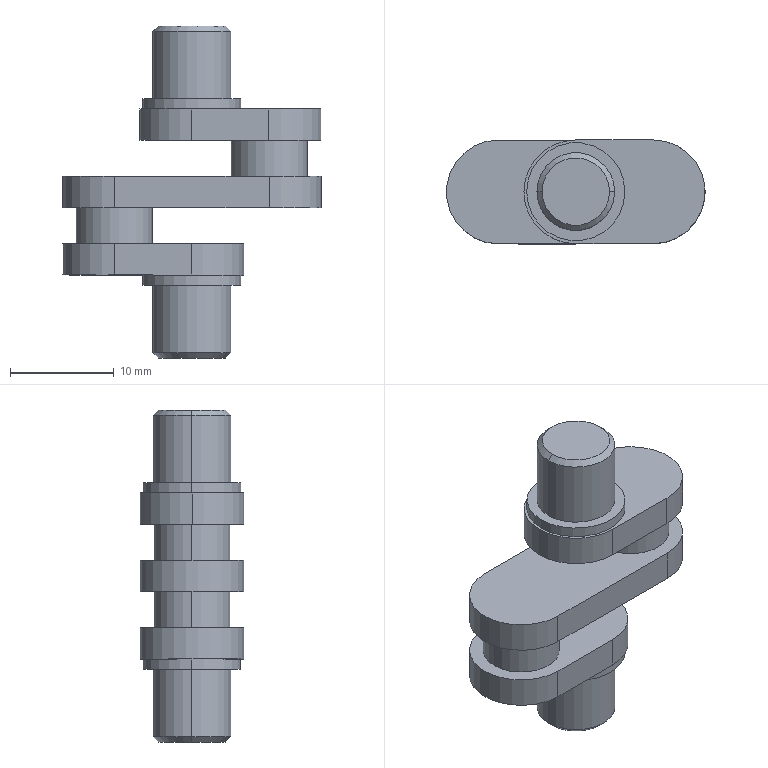Part | SolidWorks | features ICE 9, Chamfer 1 | 1 solid | 41 faces | box 24.928 x 10.008 x 32 mm | volume 2653 mm3 | cylinder 21 | plane 16 | cone 4 | commonest cylinder face diameters 10 x5 7.349 x4 7.5 x4 9.463 x4 10.004 x4
STEP:
#1=CARTESIAN_POINT('',(-3.25,0.01543,-17.5));
#2=VERTEX_POINT('',#1);
#3=CARTESIAN_POINT('',(3.25,0.01543,-17.5));
#4=VERTEX_POINT('',#3);
#5=CARTESIAN_POINT('',(0.000000001,0.01543,-17.5));
#6=DIRECTION('',(0.,0.,-1.));
#7=DIRECTION('',(-1.,0.,0.));
#8=AXIS2_PLACEMENT_3D('',#5,#6,#7);
#9=CIRCLE('',#8,3.25);
#10=EDGE_CURVE('',#2,#4,#9,.T.);
#11=ORIENTED_EDGE('',*,*,#10,.F.);
#12=CARTESIAN_POINT('',(-3.75,0.01543,-17.));
#13=VERTEX_POINT('',#12);
#14=CARTESIAN_POINT('',(-3.25,0.01543,-17.5));
#15=DIRECTION('',(-0.7071,0.,0.7071));
#16=VECTOR('',#15,1000.);
#17=LINE('',#14,#16);
#18=EDGE_CURVE('',#2,#13,#17,.T.);
#19=ORIENTED_EDGE('',*,*,#18,.T.);
#20=CARTESIAN_POINT('',(3.75,0.01543,-17.));
#21=VERTEX_POINT('',#20);
#22=CARTESIAN_POINT('',(0.000000001,0.01543,-17.));
#23=DIRECTION('',(0.,0.,1.));
#24=DIRECTION('',(-1.,0.,0.));
#25=AXIS2_PLACEMENT_3D('',#22,#23,#24);
#26=CIRCLE('',#25,3.75);
#27=EDGE_CURVE('',#21,#13,#26,.T.);
#28=ORIENTED_EDGE('',*,*,#27,.F.);
#29=CARTESIAN_POINT('',(3.25,0.01543,-17.5));
#30=DIRECTION('',(0.7071,0.,0.7071));
#31=VECTOR('',#30,1000.);
#32=LINE('',#29,#31);
#33=EDGE_CURVE('',#4,#21,#32,.T.);
#34=ORIENTED_EDGE('',*,*,#33,.F.);
#35=EDGE_LOOP('',(#11,#19,#28,#34));
#36=FACE_OUTER_BOUND('',#35,.T.);
#37=CARTESIAN_POINT('',(0.000000001,0.01543,-17.5));
#38=DIRECTION('',(0.,0.,1.));
#39=DIRECTION('',(1.,0.,0.));
#40=AXIS2_PLACEMENT_3D('',#37,#38,#39);
#41=CONICAL_SURFACE('',#40,3.25,0.7854);
#42=ADVANCED_FACE('',(#36),#41,.T.);
#43=CARTESIAN_POINT('',(3.25,0.01543,14.5));
#44=VERTEX_POINT('',#43);
#45=CARTESIAN_POINT('',(-3.25,0.01543,14.5));
#46=VERTEX_POINT('',#45);
#47=CARTESIAN_POINT('',(0.000000001,0.01543,14.5));
#48=DIRECTION('',(0.,0.,1.));
#49=DIRECTION('',(1.,0.,0.));
#50=AXIS2_PLACEMENT_3D('',#47,#48,#49);
#51=CIRCLE('',#50,3.25);
#52=EDGE_CURVE('',#44,#46,#51,.T.);
#53=ORIENTED_EDGE('',*,*,#52,.F.);
#54=CARTESIAN_POINT('',(3.75,0.01543,14.));
#55=VERTEX_POINT('',#54);
#56=CARTESIAN_POINT('',(3.25,0.01543,14.5));
#57=DIRECTION('',(0.7071,0.,-0.7071));
#58=VECTOR('',#57,1000.);
#59=LINE('',#56,#58);
#60=EDGE_CURVE('',#44,#55,#59,.T.);
#61=ORIENTED_EDGE('',*,*,#60,.T.);
#62=CARTESIAN_POINT('',(-3.75,0.01543,14.));
#63=VERTEX_POINT('',#62);
#64=CARTESIAN_POINT('',(0.000000001,0.01543,14.));
#65=DIRECTION('',(0.,0.,-1.));
#66=DIRECTION('',(1.,0.,0.));
#67=AXIS2_PLACEMENT_3D('',#64,#65,#66);
#68=CIRCLE('',#67,3.75);
#69=EDGE_CURVE('',#63,#55,#68,.T.);
#70=ORIENTED_EDGE('',*,*,#69,.F.);
#71=CARTESIAN_POINT('',(-3.25,0.01543,14.5));
#72=DIRECTION('',(-0.7071,0.,-0.7071));
#73=VECTOR('',#72,1000.);
#74=LINE('',#71,#73);
#75=EDGE_CURVE('',#46,#63,#74,.T.);
#76=ORIENTED_EDGE('',*,*,#75,.F.);
#77=EDGE_LOOP('',(#53,#61,#70,#76));
#78=FACE_OUTER_BOUND('',#77,.T.);
#79=CARTESIAN_POINT('',(0.000000001,0.01543,14.5));
#80=DIRECTION('',(0.,0.,-1.));
#81=DIRECTION('',(-1.,0.,0.));
#82=AXIS2_PLACEMENT_3D('',#79,#80,#81);
#83=CONICAL_SURFACE('',#82,3.25,0.7854);
#84=ADVANCED_FACE('',(#78),#83,.T.);
#85=ORIENTED_EDGE('',*,*,#27,.T.);
#86=CARTESIAN_POINT('',(-3.75,0.01543,-10.5));
#87=VERTEX_POINT('',#86);
#88=CARTESIAN_POINT('',(-3.75,0.01543,-17.5));
#89=DIRECTION('',(0.,0.,1.));
#90=VECTOR('',#89,1000.);
#91=LINE('',#88,#90);
#92=EDGE_CURVE('',#13,#87,#91,.T.);
#93=ORIENTED_EDGE('',*,*,#92,.T.);
#94=CARTESIAN_POINT('',(3.75,0.01543,-10.5));
#95=VERTEX_POINT('',#94);
#96=CARTESIAN_POINT('',(0.000000001,0.01543,-10.5));
#97=DIRECTION('',(0.,0.,-1.));
#98=DIRECTION('',(-1.,0.,0.));
#99=AXIS2_PLACEMENT_3D('',#96,#97,#98);
#100=CIRCLE('',#99,3.75);
#101=EDGE_CURVE('',#87,#95,#100,.T.);
#102=ORIENTED_EDGE('',*,*,#101,.T.);
#103=CARTESIAN_POINT('',(3.75,0.01543,-17.5));
#104=DIRECTION('',(0.,0.,1.));
#105=VECTOR('',#104,1000.);
#106=LINE('',#103,#105);
#107=EDGE_CURVE('',#21,#95,#106,.T.);
#108=ORIENTED_EDGE('',*,*,#107,.F.);
#109=EDGE_LOOP('',(#85,#93,#102,#108));
#110=FACE_OUTER_BOUND('',#109,.T.);
#111=CARTESIAN_POINT('',(0.000000001,0.01543,-17.5));
#112=DIRECTION('',(0.,0.,1.));
#113=DIRECTION('',(1.,0.,0.));
#114=AXIS2_PLACEMENT_3D('',#111,#112,#113);
#115=CYLINDRICAL_SURFACE('',#114,3.75);
#116=ADVANCED_FACE('',(#110),#115,.T.);
#117=CARTESIAN_POINT('',(-4.731,0.01543,-10.5));
#118=VERTEX_POINT('',#117);
#119=CARTESIAN_POINT('',(4.731,0.01543,-10.5));
#120=VERTEX_POINT('',#119);
#121=CARTESIAN_POINT('',(0.000000001,0.01543,-10.5));
#122=DIRECTION('',(0.,0.,-1.));
#123=DIRECTION('',(-1.,0.,0.));
#124=AXIS2_PLACEMENT_3D('',#121,#122,#123);
#125=CIRCLE('',#124,4.731);
#126=EDGE_CURVE('',#118,#120,#125,.T.);
#127=ORIENTED_EDGE('',*,*,#126,.F.);
#128=CARTESIAN_POINT('',(-4.731,0.01543,-9.5));
#129=VERTEX_POINT('',#128);
#130=CARTESIAN_POINT('',(-4.731,0.01543,-10.5));
#131=DIRECTION('',(0.,0.,1.));
#132=VECTOR('',#131,1000.);
#133=LINE('',#130,#132);
#134=EDGE_CURVE('',#118,#129,#133,.T.);
#135=ORIENTED_EDGE('',*,*,#134,.T.);
#136=CARTESIAN_POINT('',(4.731,0.01543,-9.5));
#137=VERTEX_POINT('',#136);
#138=CARTESIAN_POINT('',(0.000000001,0.01543,-9.5));
#139=DIRECTION('',(0.,0.,-1.));
#140=DIRECTION('',(-1.,0.,0.));
#141=AXIS2_PLACEMENT_3D('',#138,#139,#140);
#142=CIRCLE('',#141,4.731);
#143=EDGE_CURVE('',#129,#137,#142,.T.);
#144=ORIENTED_EDGE('',*,*,#143,.T.);
#145=CARTESIAN_POINT('',(4.731,0.01543,-10.5));
#146=DIRECTION('',(0.,0.,1.));
#147=VECTOR('',#146,1000.);
#148=LINE('',#145,#147);
#149=EDGE_CURVE('',#120,#137,#148,.T.);
#150=ORIENTED_EDGE('',*,*,#149,.F.);
#151=EDGE_LOOP('',(#127,#135,#144,#150));
#152=FACE_OUTER_BOUND('',#151,.T.);
#153=CARTESIAN_POINT('',(0.000000001,0.01543,-10.5));
#154=DIRECTION('',(0.,0.,1.));
#155=DIRECTION('',(1.,0.,0.));
#156=AXIS2_PLACEMENT_3D('',#153,#154,#155);
#157=CYLINDRICAL_SURFACE('',#156,4.731);
#158=ADVANCED_FACE('',(#152),#157,.T.);
#159=ORIENTED_EDGE('',*,*,#69,.T.);
#160=CARTESIAN_POINT('',(3.75,0.01543,7.5));
#161=VERTEX_POINT('',#160);
#162=CARTESIAN_POINT('',(3.75,0.01543,14.5));
#163=DIRECTION('',(0.,0.,-1.));
#164=VECTOR('',#163,1000.);
#165=LINE('',#162,#164);
#166=EDGE_CURVE('',#55,#161,#165,.T.);
#167=ORIENTED_EDGE('',*,*,#166,.T.);
#168=CARTESIAN_POINT('',(-3.75,0.01543,7.5));
#169=VERTEX_POINT('',#168);
#170=CARTESIAN_POINT('',(0.000000001,0.01543,7.5));
#171=DIRECTION('',(0.,0.,1.));
#172=DIRECTION('',(1.,0.,0.));
#173=AXIS2_PLACEMENT_3D('',#170,#171,#172);
#174=CIRCLE('',#173,3.75);
#175=EDGE_CURVE('',#161,#169,#174,.T.);
#176=ORIENTED_EDGE('',*,*,#175,.T.);
#177=CARTESIAN_POINT('',(-3.75,0.01543,14.5));
#178=DIRECTION('',(0.,0.,-1.));
#179=VECTOR('',#178,1000.);
#180=LINE('',#177,#179);
#181=EDGE_CURVE('',#63,#169,#180,.T.);
#182=ORIENTED_EDGE('',*,*,#181,.F.);
#183=EDGE_LOOP('',(#159,#167,#176,#182));
#184=FACE_OUTER_BOUND('',#183,.T.);
#185=CARTESIAN_POINT('',(0.000000001,0.01543,14.5));
#186=DIRECTION('',(0.,0.,-1.));
#187=DIRECTION('',(-1.,0.,0.));
#188=AXIS2_PLACEMENT_3D('',#185,#186,#187);
#189=CYLINDRICAL_SURFACE('',#188,3.75);
#190=ADVANCED_FACE('',(#184),#189,.T.);
#191=CARTESIAN_POINT('',(4.731,0.01543,7.5));
#192=VERTEX_POINT('',#191);
#193=CARTESIAN_POINT('',(-4.731,0.01543,7.5));
#194=VERTEX_POINT('',#193);
#195=CARTESIAN_POINT('',(0.000000001,0.01543,7.5));
#196=DIRECTION('',(0.,0.,1.));
#197=DIRECTION('',(1.,0.,0.));
#198=AXIS2_PLACEMENT_3D('',#195,#196,#197);
#199=CIRCLE('',#198,4.731);
#200=EDGE_CURVE('',#192,#194,#199,.T.);
#201=ORIENTED_EDGE('',*,*,#200,.F.);
#202=CARTESIAN_POINT('',(4.731,0.01543,6.5));
#203=VERTEX_POINT('',#202);
#204=CARTESIAN_POINT('',(4.731,0.01543,7.5));
#205=DIRECTION('',(0.,0.,-1.));
#206=VECTOR('',#205,1000.);
#207=LINE('',#204,#206);
#208=EDGE_CURVE('',#192,#203,#207,.T.);
#209=ORIENTED_EDGE('',*,*,#208,.T.);
#210=CARTESIAN_POINT('',(-4.731,0.01543,6.5));
#211=VERTEX_POINT('',#210);
#212=CARTESIAN_POINT('',(0.000000001,0.01543,6.5));
#213=DIRECTION('',(0.,0.,1.));
#214=DIRECTION('',(1.,0.,0.));
#215=AXIS2_PLACEMENT_3D('',#212,#213,#214);
#216=CIRCLE('',#215,4.731);
#217=EDGE_CURVE('',#203,#211,#216,.T.);
#218=ORIENTED_EDGE('',*,*,#217,.T.);
#219=CARTESIAN_POINT('',(-4.731,0.01543,7.5));
#220=DIRECTION('',(0.,0.,-1.));
#221=VECTOR('',#220,1000.);
#222=LINE('',#219,#221);
#223=EDGE_CURVE('',#194,#211,#222,.T.);
#224=ORIENTED_EDGE('',*,*,#223,.F.);
#225=EDGE_LOOP('',(#201,#209,#218,#224));
#226=FACE_OUTER_BOUND('',#225,.T.);
#227=CARTESIAN_POINT('',(0.000000001,0.01543,7.5));
#228=DIRECTION('',(0.,0.,-1.));
#229=DIRECTION('',(-1.,0.,0.));
#230=AXIS2_PLACEMENT_3D('',#227,#228,#229);
#231=CYLINDRICAL_SURFACE('',#230,4.731);
#232=ADVANCED_FACE('',(#226),#231,.T.);
#233=CARTESIAN_POINT('',(-5.003,0.001927,6.5));
#234=VERTEX_POINT('',#233);
#235=CARTESIAN_POINT('',(0.004312,-5.,6.5));
#236=VERTEX_POINT('',#235);
#237=CARTESIAN_POINT('',(-0.00129,0.001927,6.5));
#238=DIRECTION('',(0.,0.,1.));
#239=DIRECTION('',(1.,0.,0.));
#240=AXIS2_PLACEMENT_3D('',#237,#238,#239);
#241=CIRCLE('',#240,5.002);
#242=EDGE_CURVE('',#234,#236,#241,.T.);
#243=ORIENTED_EDGE('',*,*,#242,.F.);
#244=CARTESIAN_POINT('',(-5.003,0.001927,3.5));
#245=VERTEX_POINT('',#244);
#246=CARTESIAN_POINT('',(-5.003,0.001927,6.5));
#247=DIRECTION('',(0.,0.,-1.));
#248=VECTOR('',#247,1000.);
#249=LINE('',#246,#248);
#250=EDGE_CURVE('',#234,#245,#249,.T.);
#251=ORIENTED_EDGE('',*,*,#250,.T.);
#252=CARTESIAN_POINT('',(0.004312,-5.,3.5));
#253=VERTEX_POINT('',#252);
#254=CARTESIAN_POINT('',(-0.00129,0.001927,3.5));
#255=DIRECTION('',(0.,0.,1.));
#256=DIRECTION('',(1.,0.,0.));
#257=AXIS2_PLACEMENT_3D('',#254,#255,#256);
#258=CIRCLE('',#257,5.002);
#259=EDGE_CURVE('',#245,#253,#258,.T.);
#260=ORIENTED_EDGE('',*,*,#259,.T.);
#261=CARTESIAN_POINT('',(0.004312,-5.,6.5));
#262=DIRECTION('',(0.,0.,-1.));
#263=VECTOR('',#262,1000.);
#264=LINE('',#261,#263);
#265=EDGE_CURVE('',#236,#253,#264,.T.);
#266=ORIENTED_EDGE('',*,*,#265,.F.);
#267=EDGE_LOOP('',(#243,#251,#260,#266));
#268=FACE_OUTER_BOUND('',#267,.T.);
#269=CARTESIAN_POINT('',(-0.00129,0.001927,6.5));
#270=DIRECTION('',(0.,0.,-1.));
#271=DIRECTION('',(-1.,0.,0.));
#272=AXIS2_PLACEMENT_3D('',#269,#270,#271);
#273=CYLINDRICAL_SURFACE('',#272,5.002);
#274=ADVANCED_FACE('',(#268),#273,.T.);
#275=CARTESIAN_POINT('',(5.003,0.001927,-9.5));
#276=VERTEX_POINT('',#275);
#277=CARTESIAN_POINT('',(-0.00388,-5.,-9.5));
#278=VERTEX_POINT('',#277);
#279=CARTESIAN_POINT('',(0.001291,0.001927,-9.5));
#280=DIRECTION('',(0.,0.,-1.));
#281=DIRECTION('',(-1.,0.,0.));
#282=AXIS2_PLACEMENT_3D('',#279,#280,#281);
#283=CIRCLE('',#282,5.002);
#284=EDGE_CURVE('',#276,#278,#283,.T.);
#285=ORIENTED_EDGE('',*,*,#284,.F.);
#286=CARTESIAN_POINT('',(5.003,0.001927,-6.5));
#287=VERTEX_POINT('',#286);
#288=CARTESIAN_POINT('',(5.003,0.001927,-9.5));
#289=DIRECTION('',(0.,0.,1.));
#290=VECTOR('',#289,1000.);
#291=LINE('',#288,#290);
#292=EDGE_CURVE('',#276,#287,#291,.T.);
#293=ORIENTED_EDGE('',*,*,#292,.T.);
#294=CARTESIAN_POINT('',(-0.00388,-5.,-6.5));
#295=VERTEX_POINT('',#294);
#296=CARTESIAN_POINT('',(0.001291,0.001927,-6.5));
#297=DIRECTION('',(0.,0.,-1.));
#298=DIRECTION('',(-1.,0.,0.));
#299=AXIS2_PLACEMENT_3D('',#296,#297,#298);
#300=CIRCLE('',#299,5.002);
#301=EDGE_CURVE('',#287,#295,#300,.T.);
#302=ORIENTED_EDGE('',*,*,#301,.T.);
#303=CARTESIAN_POINT('',(-0.00388,-5.,-9.5));
#304=DIRECTION('',(0.,0.,1.));
#305=VECTOR('',#304,1000.);
#306=LINE('',#303,#305);
#307=EDGE_CURVE('',#278,#295,#306,.T.);
#308=ORIENTED_EDGE('',*,*,#307,.F.);
#309=EDGE_LOOP('',(#285,#293,#302,#308));
#310=FACE_OUTER_BOUND('',#309,.T.);
#311=CARTESIAN_POINT('',(0.001291,0.001927,-9.5));
#312=DIRECTION('',(0.,0.,1.));
#313=DIRECTION('',(1.,0.,0.));
#314=AXIS2_PLACEMENT_3D('',#311,#312,#313);
#315=CYLINDRICAL_SURFACE('',#314,5.002);
#316=ADVANCED_FACE('',(#310),#315,.T.);
#317=CARTESIAN_POINT('',(11.139,0.007713,3.5));
#318=VERTEX_POINT('',#317);
#319=CARTESIAN_POINT('',(3.789,0.007713,3.5));
#320=VERTEX_POINT('',#319);
#321=CARTESIAN_POINT('',(7.464,0.007713,3.5));
#322=DIRECTION('',(0.,0.,1.));
#323=DIRECTION('',(1.,0.,0.));
#324=AXIS2_PLACEMENT_3D('',#321,#322,#323);
#325=CIRCLE('',#324,3.675);
#326=EDGE_CURVE('',#318,#320,#325,.T.);
#327=ORIENTED_EDGE('',*,*,#326,.F.);
#328=CARTESIAN_POINT('',(11.139,0.007713,0.));
#329=VERTEX_POINT('',#328);
#330=CARTESIAN_POINT('',(11.139,0.007713,13.893));
#331=DIRECTION('',(0.,0.,-1.));
#332=VECTOR('',#331,1000.);
#333=LINE('',#330,#332);
#334=EDGE_CURVE('',#318,#329,#333,.T.);
#335=ORIENTED_EDGE('',*,*,#334,.T.);
#336=CARTESIAN_POINT('',(3.789,0.007713,0.));
#337=VERTEX_POINT('',#336);
#338=CARTESIAN_POINT('',(7.464,0.007713,0.));
#339=DIRECTION('',(0.,0.,1.));
#340=DIRECTION('',(1.,0.,0.));
#341=AXIS2_PLACEMENT_3D('',#338,#339,#340);
#342=CIRCLE('',#341,3.675);
#343=EDGE_CURVE('',#329,#337,#342,.T.);
#344=ORIENTED_EDGE('',*,*,#343,.T.);
#345=CARTESIAN_POINT('',(3.789,0.007713,13.893));
#346=DIRECTION('',(0.,0.,-1.));
#347=VECTOR('',#346,1000.);
#348=LINE('',#345,#347);
#349=EDGE_CURVE('',#320,#337,#348,.T.);
#350=ORIENTED_EDGE('',*,*,#349,.F.);
#351=EDGE_LOOP('',(#327,#335,#344,#350));
#352=FACE_OUTER_BOUND('',#351,.T.);
#353=CARTESIAN_POINT('',(7.464,0.007713,13.893));
#354=DIRECTION('',(0.,0.,-1.));
#355=DIRECTION('',(-1.,0.,0.));
#356=AXIS2_PLACEMENT_3D('',#353,#354,#355);
#357=CYLINDRICAL_SURFACE('',#356,3.675);
#358=ADVANCED_FACE('',(#352),#357,.T.);
#359=CARTESIAN_POINT('',(-3.789,0.007713,-6.5));
#360=VERTEX_POINT('',#359);
#361=CARTESIAN_POINT('',(-11.139,0.007713,-6.5));
#362=VERTEX_POINT('',#361);
#363=CARTESIAN_POINT('',(-7.464,0.007713,-6.5));
#364=DIRECTION('',(0.,0.,1.));
#365=DIRECTION('',(1.,0.,0.));
#366=AXIS2_PLACEMENT_3D('',#363,#364,#365);
#367=CIRCLE('',#366,3.675);
#368=EDGE_CURVE('',#360,#362,#367,.T.);
#369=ORIENTED_EDGE('',*,*,#368,.T.);
#370=CARTESIAN_POINT('',(-11.139,0.007713,-3.));
#371=VERTEX_POINT('',#370);
#372=CARTESIAN_POINT('',(-11.139,0.007713,-16.893));
#373=DIRECTION('',(0.,0.,1.));
#374=VECTOR('',#373,1000.);
#375=LINE('',#372,#374);
#376=EDGE_CURVE('',#362,#371,#375,.T.);
#377=ORIENTED_EDGE('',*,*,#376,.T.);
#378=CARTESIAN_POINT('',(-3.789,0.007713,-3.));
#379=VERTEX_POINT('',#378);
#380=CARTESIAN_POINT('',(-7.464,0.007713,-3.));
#381=DIRECTION('',(0.,0.,-1.));
#382=DIRECTION('',(1.,0.,0.));
#383=AXIS2_PLACEMENT_3D('',#380,#381,#382);
#384=CIRCLE('',#383,3.675);
#385=EDGE_CURVE('',#371,#379,#384,.T.);
#386=ORIENTED_EDGE('',*,*,#385,.T.);
#387=CARTESIAN_POINT('',(-3.789,0.007713,-16.893));
#388=DIRECTION('',(0.,0.,1.));
#389=VECTOR('',#388,1000.);
#390=LINE('',#387,#389);
#391=EDGE_CURVE('',#360,#379,#390,.T.);
#392=ORIENTED_EDGE('',*,*,#391,.F.);
#393=EDGE_LOOP('',(#369,#377,#386,#392));
#394=FACE_OUTER_BOUND('',#393,.T.);
#395=CARTESIAN_POINT('',(-7.464,0.007713,-16.893));
#396=DIRECTION('',(0.,0.,1.));
#397=DIRECTION('',(1.,0.,0.));
#398=AXIS2_PLACEMENT_3D('',#395,#396,#397);
#399=CYLINDRICAL_SURFACE('',#398,3.675);
#400=ADVANCED_FACE('',(#394),#399,.T.);
#401=CARTESIAN_POINT('',(12.464,0.007713,-3.));
#402=VERTEX_POINT('',#401);
#403=CARTESIAN_POINT('',(7.464,-4.992,-3.));
#404=VERTEX_POINT('',#403);
#405=CARTESIAN_POINT('',(7.464,0.007713,-3.));
#406=DIRECTION('',(0.,0.,-1.));
#407=DIRECTION('',(1.,0.,0.));
#408=AXIS2_PLACEMENT_3D('',#405,#406,#407);
#409=CIRCLE('',#408,5.);
#410=EDGE_CURVE('',#402,#404,#409,.T.);
#411=ORIENTED_EDGE('',*,*,#410,.F.);
#412=CARTESIAN_POINT('',(12.464,0.007713,0.));
#413=VERTEX_POINT('',#412);
#414=CARTESIAN_POINT('',(12.464,0.007713,-29.859));
#415=DIRECTION('',(0.,0.,1.));
#416=VECTOR('',#415,1000.);
#417=LINE('',#414,#416);
#418=EDGE_CURVE('',#402,#413,#417,.T.);
#419=ORIENTED_EDGE('',*,*,#418,.T.);
#420=CARTESIAN_POINT('',(7.464,-4.992,0.));
#421=VERTEX_POINT('',#420);
#422=CARTESIAN_POINT('',(7.464,0.007713,0.));
#423=DIRECTION('',(0.,0.,1.));
#424=DIRECTION('',(1.,0.,0.));
#425=AXIS2_PLACEMENT_3D('',#422,#423,#424);
#426=CIRCLE('',#425,5.);
#427=EDGE_CURVE('',#421,#413,#426,.T.);
#428=ORIENTED_EDGE('',*,*,#427,.F.);
#429=CARTESIAN_POINT('',(7.464,-4.992,-29.859));
#430=DIRECTION('',(0.,0.,1.));
#431=VECTOR('',#430,1000.);
#432=LINE('',#429,#431);
#433=EDGE_CURVE('',#404,#421,#432,.T.);
#434=ORIENTED_EDGE('',*,*,#433,.F.);
#435=EDGE_LOOP('',(#411,#419,#428,#434));
#436=FACE_OUTER_BOUND('',#435,.T.);
#437=CARTESIAN_POINT('',(7.464,0.007713,-29.859));
#438=DIRECTION('',(0.,0.,1.));
#439=DIRECTION('',(1.,0.,0.));
#440=AXIS2_PLACEMENT_3D('',#437,#438,#439);
#441=CYLINDRICAL_SURFACE('',#440,5.);
#442=ADVANCED_FACE('',(#436),#441,.T.);
#443=CARTESIAN_POINT('',(-7.464,-4.992,-3.));
#444=VERTEX_POINT('',#443);
#445=CARTESIAN_POINT('',(-7.464,5.008,-3.));
#446=VERTEX_POINT('',#445);
#447=CARTESIAN_POINT('',(-7.464,0.007713,-3.));
#448=DIRECTION('',(0.,0.,-1.));
#449=DIRECTION('',(1.,0.,0.));
#450=AXIS2_PLACEMENT_3D('',#447,#448,#449);
#451=CIRCLE('',#450,5.);
#452=EDGE_CURVE('',#444,#446,#451,.T.);
#453=ORIENTED_EDGE('',*,*,#452,.F.);
#454=CARTESIAN_POINT('',(-7.464,-4.992,0.));
#455=VERTEX_POINT('',#454);
#456=CARTESIAN_POINT('',(-7.464,-4.992,-29.859));
#457=DIRECTION('',(0.,0.,1.));
#458=VECTOR('',#457,1000.);
#459=LINE('',#456,#458);
#460=EDGE_CURVE('',#444,#455,#459,.T.);
#461=ORIENTED_EDGE('',*,*,#460,.T.);
#462=CARTESIAN_POINT('',(-7.464,5.008,0.));
#463=VERTEX_POINT('',#462);
#464=CARTESIAN_POINT('',(-7.464,0.007713,0.));
#465=DIRECTION('',(0.,0.,1.));
#466=DIRECTION('',(1.,0.,0.));
#467=AXIS2_PLACEMENT_3D('',#464,#465,#466);
#468=CIRCLE('',#467,5.);
#469=EDGE_CURVE('',#463,#455,#468,.T.);
#470=ORIENTED_EDGE('',*,*,#469,.F.);
#471=CARTESIAN_POINT('',(-7.464,5.008,-29.859));
#472=DIRECTION('',(0.,0.,1.));
#473=VECTOR('',#472,1000.);
#474=LINE('',#471,#473);
#475=EDGE_CURVE('',#446,#463,#474,.T.);
#476=ORIENTED_EDGE('',*,*,#475,.F.);
#477=EDGE_LOOP('',(#453,#461,#470,#476));
#478=FACE_OUTER_BOUND('',#477,.T.);
#479=CARTESIAN_POINT('',(-7.464,0.007713,-29.859));
#480=DIRECTION('',(0.,0.,1.));
#481=DIRECTION('',(1.,0.,0.));
#482=AXIS2_PLACEMENT_3D('',#479,#480,#481);
#483=CYLINDRICAL_SURFACE('',#482,5.);
#484=ADVANCED_FACE('',(#478),#483,.T.);
#485=CARTESIAN_POINT('',(7.464,5.008,-3.));
#486=VERTEX_POINT('',#485);
#487=CARTESIAN_POINT('',(-7.464,5.008,-3.));
#488=DIRECTION('',(1.,0.,0.));
#489=VECTOR('',#488,1000.);
#490=LINE('',#487,#489);
#491=EDGE_CURVE('',#446,#486,#490,.T.);
#492=ORIENTED_EDGE('',*,*,#491,.F.);
#493=ORIENTED_EDGE('',*,*,#475,.T.);
#494=CARTESIAN_POINT('',(7.464,5.008,0.));
#495=VERTEX_POINT('',#494);
#496=CARTESIAN_POINT('',(-7.464,5.008,0.));
#497=DIRECTION('',(-1.,0.,0.));
#498=VECTOR('',#497,1000.);
#499=LINE('',#496,#498);
#500=EDGE_CURVE('',#495,#463,#499,.T.);
#501=ORIENTED_EDGE('',*,*,#500,.F.);
#502=CARTESIAN_POINT('',(7.464,5.008,-29.859));
#503=DIRECTION('',(0.,0.,1.));
#504=VECTOR('',#503,1000.);
#505=LINE('',#502,#504);
#506=EDGE_CURVE('',#486,#495,#505,.T.);
#507=ORIENTED_EDGE('',*,*,#506,.F.);
#508=EDGE_LOOP('',(#492,#493,#501,#507));
#509=FACE_OUTER_BOUND('',#508,.T.);
#510=CARTESIAN_POINT('',(-7.464,5.008,-29.859));
#511=DIRECTION('',(0.,1.,0.));
#512=DIRECTION('',(0.,0.,1.));
#513=AXIS2_PLACEMENT_3D('',#510,#511,#512);
#514=PLANE('',#513);
#515=ADVANCED_FACE('',(#509),#514,.T.);
#516=ORIENTED_EDGE('',*,*,#418,.F.);
#517=CARTESIAN_POINT('',(7.464,0.007713,-3.));
#518=DIRECTION('',(0.,0.,-1.));
#519=DIRECTION('',(1.,0.,0.));
#520=AXIS2_PLACEMENT_3D('',#517,#518,#519);
#521=CIRCLE('',#520,5.);
#522=EDGE_CURVE('',#486,#402,#521,.T.);
#523=ORIENTED_EDGE('',*,*,#522,.F.);
#524=ORIENTED_EDGE('',*,*,#506,.T.);
#525=CARTESIAN_POINT('',(7.464,0.007713,0.));
#526=DIRECTION('',(0.,0.,1.));
#527=DIRECTION('',(1.,0.,0.));
#528=AXIS2_PLACEMENT_3D('',#525,#526,#527);
#529=CIRCLE('',#528,5.);
#530=EDGE_CURVE('',#413,#495,#529,.T.);
#531=ORIENTED_EDGE('',*,*,#530,.F.);
#532=EDGE_LOOP('',(#516,#523,#524,#531));
#533=FACE_OUTER_BOUND('',#532,.T.);
#534=CARTESIAN_POINT('',(7.464,0.007713,-29.859));
#535=DIRECTION('',(0.,0.,1.));
#536=DIRECTION('',(1.,0.,0.));
#537=AXIS2_PLACEMENT_3D('',#534,#535,#536);
#538=CYLINDRICAL_SURFACE('',#537,5.);
#539=ADVANCED_FACE('',(#533),#538,.T.);
#540=CARTESIAN_POINT('',(-7.464,-4.992,-3.));
#541=DIRECTION('',(-1.,-0.000000089,0.));
#542=VECTOR('',#541,1000.);
#543=LINE('',#540,#542);
#544=EDGE_CURVE('',#404,#444,#543,.T.);
#545=ORIENTED_EDGE('',*,*,#544,.F.);
#546=ORIENTED_EDGE('',*,*,#433,.T.);
#547=CARTESIAN_POINT('',(-7.464,-4.992,0.));
#548=DIRECTION('',(1.,0.000000089,0.));
#549=VECTOR('',#548,1000.);
#550=LINE('',#547,#549);
#551=EDGE_CURVE('',#455,#421,#550,.T.);
#552=ORIENTED_EDGE('',*,*,#551,.F.);
#553=ORIENTED_EDGE('',*,*,#460,.F.);
#554=EDGE_LOOP('',(#545,#546,#552,#553));
#555=FACE_OUTER_BOUND('',#554,.T.);
#556=CARTESIAN_POINT('',(-7.464,-4.992,-29.859));
#557=DIRECTION('',(0.000000089,-1.,0.));
#558=DIRECTION('',(1.,0.000000089,0.));
#559=AXIS2_PLACEMENT_3D('',#556,#557,#558);
#560=PLANE('',#559);
#561=ADVANCED_FACE('',(#555),#560,.T.);
#562=CARTESIAN_POINT('',(7.464,0.007713,0.));
#563=DIRECTION('',(0.,0.,1.));
#564=DIRECTION('',(1.,0.,0.));
#565=AXIS2_PLACEMENT_3D('',#562,#563,#564);
#566=CIRCLE('',#565,3.675);
#567=EDGE_CURVE('',#337,#329,#566,.T.);
#568=ORIENTED_EDGE('',*,*,#567,.F.);
#569=ORIENTED_EDGE('',*,*,#343,.F.);
#570=EDGE_LOOP('',(#568,#569));
#571=FACE_BOUND('',#570,.T.);
#572=ORIENTED_EDGE('',*,*,#469,.T.);
#573=ORIENTED_EDGE('',*,*,#551,.T.);
#574=ORIENTED_EDGE('',*,*,#427,.T.);
#575=ORIENTED_EDGE('',*,*,#530,.T.);
#576=ORIENTED_EDGE('',*,*,#500,.T.);
#577=EDGE_LOOP('',(#572,#573,#574,#575,#576));
#578=FACE_OUTER_BOUND('',#577,.T.);
#579=CARTESIAN_POINT('',(-7.464,0.007713,0.));
#580=DIRECTION('',(0.,0.,1.));
#581=DIRECTION('',(1.,0.,0.));
#582=AXIS2_PLACEMENT_3D('',#579,#580,#581);
#583=PLANE('',#582);
#584=ADVANCED_FACE('',(#571,#578),#583,.T.);
#585=CARTESIAN_POINT('',(-7.464,0.007713,-3.));
#586=DIRECTION('',(0.,0.,-1.));
#587=DIRECTION('',(1.,0.,0.));
#588=AXIS2_PLACEMENT_3D('',#585,#586,#587);
#589=CIRCLE('',#588,3.675);
#590=EDGE_CURVE('',#379,#371,#589,.T.);
#591=ORIENTED_EDGE('',*,*,#590,.F.);
#592=ORIENTED_EDGE('',*,*,#385,.F.);
#593=EDGE_LOOP('',(#591,#592));
#594=FACE_BOUND('',#593,.T.);
#595=ORIENTED_EDGE('',*,*,#452,.T.);
#596=ORIENTED_EDGE('',*,*,#491,.T.);
#597=ORIENTED_EDGE('',*,*,#522,.T.);
#598=ORIENTED_EDGE('',*,*,#410,.T.);
#599=ORIENTED_EDGE('',*,*,#544,.T.);
#600=EDGE_LOOP('',(#595,#596,#597,#598,#599));
#601=FACE_OUTER_BOUND('',#600,.T.);
#602=CARTESIAN_POINT('',(-34.483,1.603,-3.));
#603=DIRECTION('',(0.,0.,1.));
#604=DIRECTION('',(0.9983,-0.05894,0.));
#605=AXIS2_PLACEMENT_3D('',#602,#603,#604);
#606=PLANE('',#605);
#607=ADVANCED_FACE('',(#594,#601),#606,.F.);
#608=ORIENTED_EDGE('',*,*,#376,.F.);
#609=CARTESIAN_POINT('',(-7.464,0.007713,-6.5));
#610=DIRECTION('',(0.,0.,1.));
#611=DIRECTION('',(1.,0.,0.));
#612=AXIS2_PLACEMENT_3D('',#609,#610,#611);
#613=CIRCLE('',#612,3.675);
#614=EDGE_CURVE('',#362,#360,#613,.T.);
#615=ORIENTED_EDGE('',*,*,#614,.T.);
#616=ORIENTED_EDGE('',*,*,#391,.T.);
#617=ORIENTED_EDGE('',*,*,#590,.T.);
#618=EDGE_LOOP('',(#608,#615,#616,#617));
#619=FACE_OUTER_BOUND('',#618,.T.);
#620=CARTESIAN_POINT('',(-7.464,0.007713,-16.893));
#621=DIRECTION('',(0.,0.,1.));
#622=DIRECTION('',(1.,0.,0.));
#623=AXIS2_PLACEMENT_3D('',#620,#621,#622);
#624=CYLINDRICAL_SURFACE('',#623,3.675);
#625=ADVANCED_FACE('',(#619),#624,.T.);
#626=ORIENTED_EDGE('',*,*,#334,.F.);
#627=CARTESIAN_POINT('',(7.464,0.007713,3.5));
#628=DIRECTION('',(0.,0.,1.));
#629=DIRECTION('',(1.,0.,0.));
#630=AXIS2_PLACEMENT_3D('',#627,#628,#629);
#631=CIRCLE('',#630,3.675);
#632=EDGE_CURVE('',#320,#318,#631,.T.);
#633=ORIENTED_EDGE('',*,*,#632,.F.);
#634=ORIENTED_EDGE('',*,*,#349,.T.);
#635=ORIENTED_EDGE('',*,*,#567,.T.);
#636=EDGE_LOOP('',(#626,#633,#634,#635));
#637=FACE_OUTER_BOUND('',#636,.T.);
#638=CARTESIAN_POINT('',(7.464,0.007713,13.893));
#639=DIRECTION('',(0.,0.,-1.));
#640=DIRECTION('',(-1.,0.,0.));
#641=AXIS2_PLACEMENT_3D('',#638,#639,#640);
#642=CYLINDRICAL_SURFACE('',#641,3.675);
#643=ADVANCED_FACE('',(#637),#642,.T.);
#644=CARTESIAN_POINT('',(0.003874,5.004,-6.5));
#645=VERTEX_POINT('',#644);
#646=CARTESIAN_POINT('',(-7.464,5.008,-6.5));
#647=VERTEX_POINT('',#646);
#648=CARTESIAN_POINT('',(0.002584,5.004,-6.5));
#649=DIRECTION('',(-1.,0.0005165,0.));
#650=VECTOR('',#649,1000.);
#651=LINE('',#648,#650);
#652=EDGE_CURVE('',#645,#647,#651,.T.);
#653=ORIENTED_EDGE('',*,*,#652,.F.);
#654=CARTESIAN_POINT('',(0.003874,5.004,-9.5));
#655=VERTEX_POINT('',#654);
#656=CARTESIAN_POINT('',(0.003874,5.004,-9.5));
#657=DIRECTION('',(0.,0.,1.));
#658=VECTOR('',#657,1000.);
#659=LINE('',#656,#658);
#660=EDGE_CURVE('',#655,#645,#659,.T.);
#661=ORIENTED_EDGE('',*,*,#660,.F.);
#662=CARTESIAN_POINT('',(-7.464,5.008,-9.5));
#663=VERTEX_POINT('',#662);
#664=CARTESIAN_POINT('',(0.002584,5.004,-9.5));
#665=DIRECTION('',(-1.,0.0005165,0.));
#666=VECTOR('',#665,1000.);
#667=LINE('',#664,#666);
#668=EDGE_CURVE('',#655,#663,#667,.T.);
#669=ORIENTED_EDGE('',*,*,#668,.T.);
#670=CARTESIAN_POINT('',(-7.464,5.008,-9.5));
#671=DIRECTION('',(0.,0.,1.));
#672=VECTOR('',#671,1000.);
#673=LINE('',#670,#672);
#674=EDGE_CURVE('',#663,#647,#673,.T.);
#675=ORIENTED_EDGE('',*,*,#674,.T.);
#676=EDGE_LOOP('',(#653,#661,#669,#675));
#677=FACE_OUTER_BOUND('',#676,.T.);
#678=CARTESIAN_POINT('',(0.002584,5.004,-9.5));
#679=DIRECTION('',(0.0005165,1.,0.));
#680=DIRECTION('',(-1.,0.0005165,0.));
#681=AXIS2_PLACEMENT_3D('',#678,#679,#680);
#682=PLANE('',#681);
#683=ADVANCED_FACE('',(#677),#682,.T.);
#684=ORIENTED_EDGE('',*,*,#292,.F.);
#685=CARTESIAN_POINT('',(0.001291,0.001927,-9.5));
#686=DIRECTION('',(0.,0.,-1.));
#687=DIRECTION('',(-1.,0.,0.));
#688=AXIS2_PLACEMENT_3D('',#685,#686,#687);
#689=CIRCLE('',#688,5.002);
#690=EDGE_CURVE('',#655,#276,#689,.T.);
#691=ORIENTED_EDGE('',*,*,#690,.F.);
#692=ORIENTED_EDGE('',*,*,#660,.T.);
#693=CARTESIAN_POINT('',(0.001291,0.001927,-6.5));
#694=DIRECTION('',(0.,0.,-1.));
#695=DIRECTION('',(-1.,0.,0.));
#696=AXIS2_PLACEMENT_3D('',#693,#694,#695);
#697=CIRCLE('',#696,5.002);
#698=EDGE_CURVE('',#645,#287,#697,.T.);
#699=ORIENTED_EDGE('',*,*,#698,.T.);
#700=EDGE_LOOP('',(#684,#691,#692,#699));
#701=FACE_OUTER_BOUND('',#700,.T.);
#702=CARTESIAN_POINT('',(0.001291,0.001927,-9.5));
#703=DIRECTION('',(0.,0.,1.));
#704=DIRECTION('',(1.,0.,0.));
#705=AXIS2_PLACEMENT_3D('',#702,#703,#704);
#706=CYLINDRICAL_SURFACE('',#705,5.002);
#707=ADVANCED_FACE('',(#701),#706,.T.);
#708=CARTESIAN_POINT('',(-7.464,-4.992,-6.5));
#709=VERTEX_POINT('',#708);
#710=CARTESIAN_POINT('',(-0.005169,-5.,-6.5));
#711=DIRECTION('',(-1.,0.001034,0.));
#712=VECTOR('',#711,1000.);
#713=LINE('',#710,#712);
#714=EDGE_CURVE('',#295,#709,#713,.T.);
#715=ORIENTED_EDGE('',*,*,#714,.T.);
#716=CARTESIAN_POINT('',(-7.464,-4.992,-9.5));
#717=VERTEX_POINT('',#716);
#718=CARTESIAN_POINT('',(-7.464,-4.992,-9.5));
#719=DIRECTION('',(0.,0.,1.));
#720=VECTOR('',#719,1000.);
#721=LINE('',#718,#720);
#722=EDGE_CURVE('',#717,#709,#721,.T.);
#723=ORIENTED_EDGE('',*,*,#722,.F.);
#724=CARTESIAN_POINT('',(-0.005169,-5.,-9.5));
#725=DIRECTION('',(-1.,0.001034,0.));
#726=VECTOR('',#725,1000.);
#727=LINE('',#724,#726);
#728=EDGE_CURVE('',#278,#717,#727,.T.);
#729=ORIENTED_EDGE('',*,*,#728,.F.);
#730=ORIENTED_EDGE('',*,*,#307,.T.);
#731=EDGE_LOOP('',(#715,#723,#729,#730));
#732=FACE_OUTER_BOUND('',#731,.T.);
#733=CARTESIAN_POINT('',(-0.005169,-5.,-9.5));
#734=DIRECTION('',(0.001034,1.,0.));
#735=DIRECTION('',(-1.,0.001034,0.));
#736=AXIS2_PLACEMENT_3D('',#733,#734,#735);
#737=PLANE('',#736);
#738=ADVANCED_FACE('',(#732),#737,.F.);
#739=CARTESIAN_POINT('',(-7.464,0.007713,-6.5));
#740=DIRECTION('',(0.,0.,-1.));
#741=DIRECTION('',(-1.,0.,0.));
#742=AXIS2_PLACEMENT_3D('',#739,#740,#741);
#743=CIRCLE('',#742,5.);
#744=EDGE_CURVE('',#709,#647,#743,.T.);
#745=ORIENTED_EDGE('',*,*,#744,.T.);
#746=ORIENTED_EDGE('',*,*,#674,.F.);
#747=CARTESIAN_POINT('',(-7.464,0.007713,-9.5));
#748=DIRECTION('',(0.,0.,-1.));
#749=DIRECTION('',(-1.,0.,0.));
#750=AXIS2_PLACEMENT_3D('',#747,#748,#749);
#751=CIRCLE('',#750,5.);
#752=EDGE_CURVE('',#717,#663,#751,.T.);
#753=ORIENTED_EDGE('',*,*,#752,.F.);
#754=ORIENTED_EDGE('',*,*,#722,.T.);
#755=EDGE_LOOP('',(#745,#746,#753,#754));
#756=FACE_OUTER_BOUND('',#755,.T.);
#757=CARTESIAN_POINT('',(-7.464,0.007713,-9.5));
#758=DIRECTION('',(0.,0.,1.));
#759=DIRECTION('',(1.,0.,0.));
#760=AXIS2_PLACEMENT_3D('',#757,#758,#759);
#761=CYLINDRICAL_SURFACE('',#760,5.);
#762=ADVANCED_FACE('',(#756),#761,.T.);
#763=CARTESIAN_POINT('',(0.000000001,0.01543,-9.5));
#764=DIRECTION('',(0.,0.,-1.));
#765=DIRECTION('',(-1.,0.,0.));
#766=AXIS2_PLACEMENT_3D('',#763,#764,#765);
#767=CIRCLE('',#766,4.731);
#768=EDGE_CURVE('',#137,#129,#767,.T.);
#769=ORIENTED_EDGE('',*,*,#768,.F.);
#770=ORIENTED_EDGE('',*,*,#143,.F.);
#771=EDGE_LOOP('',(#769,#770));
#772=FACE_BOUND('',#771,.T.);
#773=ORIENTED_EDGE('',*,*,#668,.F.);
#774=ORIENTED_EDGE('',*,*,#690,.T.);
#775=ORIENTED_EDGE('',*,*,#284,.T.);
#776=ORIENTED_EDGE('',*,*,#728,.T.);
#777=ORIENTED_EDGE('',*,*,#752,.T.);
#778=EDGE_LOOP('',(#773,#774,#775,#776,#777));
#779=FACE_OUTER_BOUND('',#778,.T.);
#780=CARTESIAN_POINT('',(0.,0.,-9.5));
#781=DIRECTION('',(0.,0.,-1.));
#782=DIRECTION('',(-1.,0.,0.));
#783=AXIS2_PLACEMENT_3D('',#780,#781,#782);
#784=PLANE('',#783);
#785=ADVANCED_FACE('',(#772,#779),#784,.T.);
#786=ORIENTED_EDGE('',*,*,#368,.F.);
#787=ORIENTED_EDGE('',*,*,#614,.F.);
#788=EDGE_LOOP('',(#786,#787));
#789=FACE_BOUND('',#788,.T.);
#790=ORIENTED_EDGE('',*,*,#652,.T.);
#791=ORIENTED_EDGE('',*,*,#744,.F.);
#792=ORIENTED_EDGE('',*,*,#714,.F.);
#793=ORIENTED_EDGE('',*,*,#301,.F.);
#794=ORIENTED_EDGE('',*,*,#698,.F.);
#795=EDGE_LOOP('',(#790,#791,#792,#793,#794));
#796=FACE_OUTER_BOUND('',#795,.T.);
#797=CARTESIAN_POINT('',(0.,0.,-6.5));
#798=DIRECTION('',(0.,0.,-1.));
#799=DIRECTION('',(-1.,0.,0.));
#800=AXIS2_PLACEMENT_3D('',#797,#798,#799);
#801=PLANE('',#800);
#802=ADVANCED_FACE('',(#789,#796),#801,.F.);
#803=CARTESIAN_POINT('',(-0.003874,5.004,3.5));
#804=VERTEX_POINT('',#803);
#805=CARTESIAN_POINT('',(7.464,5.008,3.5));
#806=VERTEX_POINT('',#805);
#807=CARTESIAN_POINT('',(-0.002584,5.004,3.5));
#808=DIRECTION('',(1.,0.0005165,0.));
#809=VECTOR('',#808,1000.);
#810=LINE('',#807,#809);
#811=EDGE_CURVE('',#804,#806,#810,.T.);
#812=ORIENTED_EDGE('',*,*,#811,.F.);
#813=CARTESIAN_POINT('',(-0.003874,5.004,6.5));
#814=VERTEX_POINT('',#813);
#815=CARTESIAN_POINT('',(-0.003874,5.004,6.5));
#816=DIRECTION('',(0.,0.,-1.));
#817=VECTOR('',#816,1000.);
#818=LINE('',#815,#817);
#819=EDGE_CURVE('',#814,#804,#818,.T.);
#820=ORIENTED_EDGE('',*,*,#819,.F.);
#821=CARTESIAN_POINT('',(7.464,5.008,6.5));
#822=VERTEX_POINT('',#821);
#823=CARTESIAN_POINT('',(-0.002584,5.004,6.5));
#824=DIRECTION('',(1.,0.0005165,0.));
#825=VECTOR('',#824,1000.);
#826=LINE('',#823,#825);
#827=EDGE_CURVE('',#814,#822,#826,.T.);
#828=ORIENTED_EDGE('',*,*,#827,.T.);
#829=CARTESIAN_POINT('',(7.464,5.008,6.5));
#830=DIRECTION('',(0.,0.,-1.));
#831=VECTOR('',#830,1000.);
#832=LINE('',#829,#831);
#833=EDGE_CURVE('',#822,#806,#832,.T.);
#834=ORIENTED_EDGE('',*,*,#833,.T.);
#835=EDGE_LOOP('',(#812,#820,#828,#834));
#836=FACE_OUTER_BOUND('',#835,.T.);
#837=CARTESIAN_POINT('',(-0.002584,5.004,6.5));
#838=DIRECTION('',(-0.0005165,1.,0.));
#839=DIRECTION('',(-1.,-0.0005165,0.));
#840=AXIS2_PLACEMENT_3D('',#837,#838,#839);
#841=PLANE('',#840);
#842=ADVANCED_FACE('',(#836),#841,.T.);
#843=ORIENTED_EDGE('',*,*,#250,.F.);
#844=CARTESIAN_POINT('',(-0.00129,0.001927,6.5));
#845=DIRECTION('',(0.,0.,1.));
#846=DIRECTION('',(1.,0.,0.));
#847=AXIS2_PLACEMENT_3D('',#844,#845,#846);
#848=CIRCLE('',#847,5.002);
#849=EDGE_CURVE('',#814,#234,#848,.T.);
#850=ORIENTED_EDGE('',*,*,#849,.F.);
#851=ORIENTED_EDGE('',*,*,#819,.T.);
#852=CARTESIAN_POINT('',(-0.00129,0.001927,3.5));
#853=DIRECTION('',(0.,0.,1.));
#854=DIRECTION('',(1.,0.,0.));
#855=AXIS2_PLACEMENT_3D('',#852,#853,#854);
#856=CIRCLE('',#855,5.002);
#857=EDGE_CURVE('',#804,#245,#856,.T.);
#858=ORIENTED_EDGE('',*,*,#857,.T.);
#859=EDGE_LOOP('',(#843,#850,#851,#858));
#860=FACE_OUTER_BOUND('',#859,.T.);
#861=CARTESIAN_POINT('',(-0.00129,0.001927,6.5));
#862=DIRECTION('',(0.,0.,-1.));
#863=DIRECTION('',(-1.,0.,0.));
#864=AXIS2_PLACEMENT_3D('',#861,#862,#863);
#865=CYLINDRICAL_SURFACE('',#864,5.002);
#866=ADVANCED_FACE('',(#860),#865,.T.);
#867=CARTESIAN_POINT('',(7.389,-4.992,3.5));
#868=VERTEX_POINT('',#867);
#869=CARTESIAN_POINT('',(0.0056,-5.,3.5));
#870=DIRECTION('',(1.,0.00112,0.));
#871=VECTOR('',#870,1000.);
#872=LINE('',#869,#871);
#873=EDGE_CURVE('',#253,#868,#872,.T.);
#874=ORIENTED_EDGE('',*,*,#873,.T.);
#875=CARTESIAN_POINT('',(7.389,-4.992,6.5));
#876=VERTEX_POINT('',#875);
#877=CARTESIAN_POINT('',(7.389,-4.992,6.5));
#878=DIRECTION('',(0.,0.,-1.));
#879=VECTOR('',#878,1000.);
#880=LINE('',#877,#879);
#881=EDGE_CURVE('',#876,#868,#880,.T.);
#882=ORIENTED_EDGE('',*,*,#881,.F.);
#883=CARTESIAN_POINT('',(0.0056,-5.,6.5));
#884=DIRECTION('',(1.,0.00112,0.));
#885=VECTOR('',#884,1000.);
#886=LINE('',#883,#885);
#887=EDGE_CURVE('',#236,#876,#886,.T.);
#888=ORIENTED_EDGE('',*,*,#887,.F.);
#889=ORIENTED_EDGE('',*,*,#265,.T.);
#890=EDGE_LOOP('',(#874,#882,#888,#889));
#891=FACE_OUTER_BOUND('',#890,.T.);
#892=CARTESIAN_POINT('',(0.0056,-5.,6.5));
#893=DIRECTION('',(-0.00112,1.,0.));
#894=DIRECTION('',(-1.,-0.00112,0.));
#895=AXIS2_PLACEMENT_3D('',#892,#893,#894);
#896=PLANE('',#895);
#897=ADVANCED_FACE('',(#891),#896,.F.);
#898=CARTESIAN_POINT('',(7.464,0.007713,3.5));
#899=DIRECTION('',(0.,0.,1.));
#900=DIRECTION('',(1.,0.,0.));
#901=AXIS2_PLACEMENT_3D('',#898,#899,#900);
#902=CIRCLE('',#901,5.);
#903=EDGE_CURVE('',#868,#806,#902,.T.);
#904=ORIENTED_EDGE('',*,*,#903,.T.);
#905=ORIENTED_EDGE('',*,*,#833,.F.);
#906=CARTESIAN_POINT('',(7.464,0.007713,6.5));
#907=DIRECTION('',(0.,0.,1.));
#908=DIRECTION('',(1.,0.,0.));
#909=AXIS2_PLACEMENT_3D('',#906,#907,#908);
#910=CIRCLE('',#909,5.);
#911=EDGE_CURVE('',#876,#822,#910,.T.);
#912=ORIENTED_EDGE('',*,*,#911,.F.);
#913=ORIENTED_EDGE('',*,*,#881,.T.);
#914=EDGE_LOOP('',(#904,#905,#912,#913));
#915=FACE_OUTER_BOUND('',#914,.T.);
#916=CARTESIAN_POINT('',(7.464,0.007713,6.5));
#917=DIRECTION('',(0.,0.,-1.));
#918=DIRECTION('',(-1.,0.,0.));
#919=AXIS2_PLACEMENT_3D('',#916,#917,#918);
#920=CYLINDRICAL_SURFACE('',#919,5.);
#921=ADVANCED_FACE('',(#915),#920,.T.);
#922=CARTESIAN_POINT('',(0.000000001,0.01543,6.5));
#923=DIRECTION('',(0.,0.,1.));
#924=DIRECTION('',(1.,0.,0.));
#925=AXIS2_PLACEMENT_3D('',#922,#923,#924);
#926=CIRCLE('',#925,4.731);
#927=EDGE_CURVE('',#211,#203,#926,.T.);
#928=ORIENTED_EDGE('',*,*,#927,.F.);
#929=ORIENTED_EDGE('',*,*,#217,.F.);
#930=EDGE_LOOP('',(#928,#929));
#931=FACE_BOUND('',#930,.T.);
#932=ORIENTED_EDGE('',*,*,#827,.F.);
#933=ORIENTED_EDGE('',*,*,#849,.T.);
#934=ORIENTED_EDGE('',*,*,#242,.T.);
#935=ORIENTED_EDGE('',*,*,#887,.T.);
#936=ORIENTED_EDGE('',*,*,#911,.T.);
#937=EDGE_LOOP('',(#932,#933,#934,#935,#936));
#938=FACE_OUTER_BOUND('',#937,.T.);
#939=CARTESIAN_POINT('',(0.,0.,6.5));
#940=DIRECTION('',(0.,0.,1.));
#941=DIRECTION('',(1.,0.,0.));
#942=AXIS2_PLACEMENT_3D('',#939,#940,#941);
#943=PLANE('',#942);
#944=ADVANCED_FACE('',(#931,#938),#943,.T.);
#945=ORIENTED_EDGE('',*,*,#632,.T.);
#946=ORIENTED_EDGE('',*,*,#326,.T.);
#947=EDGE_LOOP('',(#945,#946));
#948=FACE_BOUND('',#947,.T.);
#949=ORIENTED_EDGE('',*,*,#811,.T.);
#950=ORIENTED_EDGE('',*,*,#903,.F.);
#951=ORIENTED_EDGE('',*,*,#873,.F.);
#952=ORIENTED_EDGE('',*,*,#259,.F.);
#953=ORIENTED_EDGE('',*,*,#857,.F.);
#954=EDGE_LOOP('',(#949,#950,#951,#952,#953));
#955=FACE_OUTER_BOUND('',#954,.T.);
#956=CARTESIAN_POINT('',(0.,0.,3.5));
#957=DIRECTION('',(0.,0.,1.));
#958=DIRECTION('',(1.,0.,0.));
#959=AXIS2_PLACEMENT_3D('',#956,#957,#958);
#960=PLANE('',#959);
#961=ADVANCED_FACE('',(#948,#955),#960,.F.);
#962=ORIENTED_EDGE('',*,*,#208,.F.);
#963=CARTESIAN_POINT('',(0.000000001,0.01543,7.5));
#964=DIRECTION('',(0.,0.,1.));
#965=DIRECTION('',(1.,0.,0.));
#966=AXIS2_PLACEMENT_3D('',#963,#964,#965);
#967=CIRCLE('',#966,4.731);
#968=EDGE_CURVE('',#194,#192,#967,.T.);
#969=ORIENTED_EDGE('',*,*,#968,.F.);
#970=ORIENTED_EDGE('',*,*,#223,.T.);
#971=ORIENTED_EDGE('',*,*,#927,.T.);
#972=EDGE_LOOP('',(#962,#969,#970,#971));
#973=FACE_OUTER_BOUND('',#972,.T.);
#974=CARTESIAN_POINT('',(0.000000001,0.01543,7.5));
#975=DIRECTION('',(0.,0.,-1.));
#976=DIRECTION('',(-1.,0.,0.));
#977=AXIS2_PLACEMENT_3D('',#974,#975,#976);
#978=CYLINDRICAL_SURFACE('',#977,4.731);
#979=ADVANCED_FACE('',(#973),#978,.T.);
#980=CARTESIAN_POINT('',(0.000000001,0.01543,7.5));
#981=DIRECTION('',(0.,0.,1.));
#982=DIRECTION('',(1.,0.,0.));
#983=AXIS2_PLACEMENT_3D('',#980,#981,#982);
#984=CIRCLE('',#983,3.75);
#985=EDGE_CURVE('',#169,#161,#984,.T.);
#986=ORIENTED_EDGE('',*,*,#985,.F.);
#987=ORIENTED_EDGE('',*,*,#175,.F.);
#988=EDGE_LOOP('',(#986,#987));
#989=FACE_BOUND('',#988,.T.);
#990=ORIENTED_EDGE('',*,*,#968,.T.);
#991=ORIENTED_EDGE('',*,*,#200,.T.);
#992=EDGE_LOOP('',(#990,#991));
#993=FACE_OUTER_BOUND('',#992,.T.);
#994=CARTESIAN_POINT('',(0.000000001,0.01543,7.5));
#995=DIRECTION('',(0.,0.,1.));
#996=DIRECTION('',(1.,0.,0.));
#997=AXIS2_PLACEMENT_3D('',#994,#995,#996);
#998=PLANE('',#997);
#999=ADVANCED_FACE('',(#989,#993),#998,.T.);
#1000=ORIENTED_EDGE('',*,*,#166,.F.);
#1001=CARTESIAN_POINT('',(0.000000001,0.01543,14.));
#1002=DIRECTION('',(0.,0.,-1.));
#1003=DIRECTION('',(1.,0.,0.));
#1004=AXIS2_PLACEMENT_3D('',#1001,#1002,#1003);
#1005=CIRCLE('',#1004,3.75);
#1006=EDGE_CURVE('',#55,#63,#1005,.T.);
#1007=ORIENTED_EDGE('',*,*,#1006,.T.);
#1008=ORIENTED_EDGE('',*,*,#181,.T.);
#1009=ORIENTED_EDGE('',*,*,#985,.T.);
#1010=EDGE_LOOP('',(#1000,#1007,#1008,#1009));
#1011=FACE_OUTER_BOUND('',#1010,.T.);
#1012=CARTESIAN_POINT('',(0.000000001,0.01543,14.5));
#1013=DIRECTION('',(0.,0.,-1.));
#1014=DIRECTION('',(-1.,0.,0.));
#1015=AXIS2_PLACEMENT_3D('',#1012,#1013,#1014);
#1016=CYLINDRICAL_SURFACE('',#1015,3.75);
#1017=ADVANCED_FACE('',(#1011),#1016,.T.);
#1018=CARTESIAN_POINT('',(0.000000001,0.01543,14.5));
#1019=DIRECTION('',(0.,0.,1.));
#1020=DIRECTION('',(1.,0.,0.));
#1021=AXIS2_PLACEMENT_3D('',#1018,#1019,#1020);
#1022=CIRCLE('',#1021,3.25);
#1023=EDGE_CURVE('',#46,#44,#1022,.T.);
#1024=ORIENTED_EDGE('',*,*,#1023,.T.);
#1025=ORIENTED_EDGE('',*,*,#52,.T.);
#1026=EDGE_LOOP('',(#1024,#1025));
#1027=FACE_OUTER_BOUND('',#1026,.T.);
#1028=CARTESIAN_POINT('',(0.000000001,0.01543,14.5));
#1029=DIRECTION('',(0.,0.,1.));
#1030=DIRECTION('',(1.,0.,0.));
#1031=AXIS2_PLACEMENT_3D('',#1028,#1029,#1030);
#1032=PLANE('',#1031);
#1033=ADVANCED_FACE('',(#1027),#1032,.T.);
#1034=ORIENTED_EDGE('',*,*,#134,.F.);
#1035=CARTESIAN_POINT('',(0.000000001,0.01543,-10.5));
#1036=DIRECTION('',(0.,0.,-1.));
#1037=DIRECTION('',(-1.,0.,0.));
#1038=AXIS2_PLACEMENT_3D('',#1035,#1036,#1037);
#1039=CIRCLE('',#1038,4.731);
#1040=EDGE_CURVE('',#120,#118,#1039,.T.);
#1041=ORIENTED_EDGE('',*,*,#1040,.F.);
#1042=ORIENTED_EDGE('',*,*,#149,.T.);
#1043=ORIENTED_EDGE('',*,*,#768,.T.);
#1044=EDGE_LOOP('',(#1034,#1041,#1042,#1043));
#1045=FACE_OUTER_BOUND('',#1044,.T.);
#1046=CARTESIAN_POINT('',(0.000000001,0.01543,-10.5));
#1047=DIRECTION('',(0.,0.,1.));
#1048=DIRECTION('',(1.,0.,0.));
#1049=AXIS2_PLACEMENT_3D('',#1046,#1047,#1048);
#1050=CYLINDRICAL_SURFACE('',#1049,4.731);
#1051=ADVANCED_FACE('',(#1045),#1050,.T.);
#1052=CARTESIAN_POINT('',(0.000000001,0.01543,-10.5));
#1053=DIRECTION('',(0.,0.,-1.));
#1054=DIRECTION('',(-1.,0.,0.));
#1055=AXIS2_PLACEMENT_3D('',#1052,#1053,#1054);
#1056=CIRCLE('',#1055,3.75);
#1057=EDGE_CURVE('',#95,#87,#1056,.T.);
#1058=ORIENTED_EDGE('',*,*,#1057,.F.);
#1059=ORIENTED_EDGE('',*,*,#101,.F.);
#1060=EDGE_LOOP('',(#1058,#1059));
#1061=FACE_BOUND('',#1060,.T.);
#1062=ORIENTED_EDGE('',*,*,#1040,.T.);
#1063=ORIENTED_EDGE('',*,*,#126,.T.);
#1064=EDGE_LOOP('',(#1062,#1063));
#1065=FACE_OUTER_BOUND('',#1064,.T.);
#1066=CARTESIAN_POINT('',(0.000000001,0.01543,-10.5));
#1067=DIRECTION('',(0.,0.,-1.));
#1068=DIRECTION('',(-1.,0.,0.));
#1069=AXIS2_PLACEMENT_3D('',#1066,#1067,#1068);
#1070=PLANE('',#1069);
#1071=ADVANCED_FACE('',(#1061,#1065),#1070,.T.);
#1072=ORIENTED_EDGE('',*,*,#92,.F.);
#1073=CARTESIAN_POINT('',(0.000000001,0.01543,-17.));
#1074=DIRECTION('',(0.,0.,1.));
#1075=DIRECTION('',(-1.,0.,0.));
#1076=AXIS2_PLACEMENT_3D('',#1073,#1074,#1075);
#1077=CIRCLE('',#1076,3.75);
#1078=EDGE_CURVE('',#13,#21,#1077,.T.);
#1079=ORIENTED_EDGE('',*,*,#1078,.T.);
#1080=ORIENTED_EDGE('',*,*,#107,.T.);
#1081=ORIENTED_EDGE('',*,*,#1057,.T.);
#1082=EDGE_LOOP('',(#1072,#1079,#1080,#1081));
#1083=FACE_OUTER_BOUND('',#1082,.T.);
#1084=CARTESIAN_POINT('',(0.000000001,0.01543,-17.5));
#1085=DIRECTION('',(0.,0.,1.));
#1086=DIRECTION('',(1.,0.,0.));
#1087=AXIS2_PLACEMENT_3D('',#1084,#1085,#1086);
#1088=CYLINDRICAL_SURFACE('',#1087,3.75);
#1089=ADVANCED_FACE('',(#1083),#1088,.T.);
#1090=CARTESIAN_POINT('',(0.000000001,0.01543,-17.5));
#1091=DIRECTION('',(0.,0.,-1.));
#1092=DIRECTION('',(-1.,0.,0.));
#1093=AXIS2_PLACEMENT_3D('',#1090,#1091,#1092);
#1094=CIRCLE('',#1093,3.25);
#1095=EDGE_CURVE('',#4,#2,#1094,.T.);
#1096=ORIENTED_EDGE('',*,*,#1095,.T.);
#1097=ORIENTED_EDGE('',*,*,#10,.T.);
#1098=EDGE_LOOP('',(#1096,#1097));
#1099=FACE_OUTER_BOUND('',#1098,.T.);
#1100=CARTESIAN_POINT('',(0.000000001,0.01543,-17.5));
#1101=DIRECTION('',(0.,0.,-1.));
#1102=DIRECTION('',(-1.,0.,0.));
#1103=AXIS2_PLACEMENT_3D('',#1100,#1101,#1102);
#1104=PLANE('',#1103);
#1105=ADVANCED_FACE('',(#1099),#1104,.T.);
#1106=ORIENTED_EDGE('',*,*,#60,.F.);
#1107=ORIENTED_EDGE('',*,*,#1023,.F.);
#1108=ORIENTED_EDGE('',*,*,#75,.T.);
#1109=ORIENTED_EDGE('',*,*,#1006,.F.);
#1110=EDGE_LOOP('',(#1106,#1107,#1108,#1109));
#1111=FACE_OUTER_BOUND('',#1110,.T.);
#1112=CARTESIAN_POINT('',(0.000000001,0.01543,14.5));
#1113=DIRECTION('',(0.,0.,-1.));
#1114=DIRECTION('',(-1.,0.,0.));
#1115=AXIS2_PLACEMENT_3D('',#1112,#1113,#1114);
#1116=CONICAL_SURFACE('',#1115,3.25,0.7854);
#1117=ADVANCED_FACE('',(#1111),#1116,.T.);
#1118=ORIENTED_EDGE('',*,*,#18,.F.);
#1119=ORIENTED_EDGE('',*,*,#1095,.F.);
#1120=ORIENTED_EDGE('',*,*,#33,.T.);
#1121=ORIENTED_EDGE('',*,*,#1078,.F.);
#1122=EDGE_LOOP('',(#1118,#1119,#1120,#1121));
#1123=FACE_OUTER_BOUND('',#1122,.T.);
#1124=CARTESIAN_POINT('',(0.000000001,0.01543,-17.5));
#1125=DIRECTION('',(0.,0.,1.));
#1126=DIRECTION('',(1.,0.,0.));
#1127=AXIS2_PLACEMENT_3D('',#1124,#1125,#1126);
#1128=CONICAL_SURFACE('',#1127,3.25,0.7854);
#1129=ADVANCED_FACE('',(#1123),#1128,.T.);
#1130=CLOSED_SHELL('',(#42,#84,#116,#158,#190,#232,#274,#316,#358,#400,#442,#484,#515,#539,#561,#584,#607,#625,#643,#683,#707,#738,#762,#785,#802,#842,#866,#897,#921,#944,#961,#979,#999,#1017,#1033,#1051,#1071,#1089,#1105,#1117,#1129));
#1131=MANIFOLD_SOLID_BREP('',#1130);
#1132=CARTESIAN_POINT('',(0.,0.,0.));
#1133=DIRECTION('',(0.,0.,1.));
#1134=DIRECTION('',(1.,0.,0.));
#1135=AXIS2_PLACEMENT_3D('',#1132,#1133,#1134);
#1136=(LENGTH_UNIT()NAMED_UNIT(*)SI_UNIT(.MILLI.,.METRE.));
#1137=UNCERTAINTY_MEASURE_WITH_UNIT(LENGTH_MEASURE(0.00001),#1136,'','');
#1138=(NAMED_UNIT(*)PLANE_ANGLE_UNIT()SI_UNIT($,.RADIAN.));
#1139=(NAMED_UNIT(*)SI_UNIT($,.STERADIAN.)SOLID_ANGLE_UNIT());
#1140=(GEOMETRIC_REPRESENTATION_CONTEXT(3)GLOBAL_UNCERTAINTY_ASSIGNED_CONTEXT((#1137))GLOBAL_UNIT_ASSIGNED_CONTEXT((#1136,#1138,#1139))REPRESENTATION_CONTEXT('',''));
#1141=ADVANCED_BREP_SHAPE_REPRESENTATION('',(#1131,#1135),#1140);